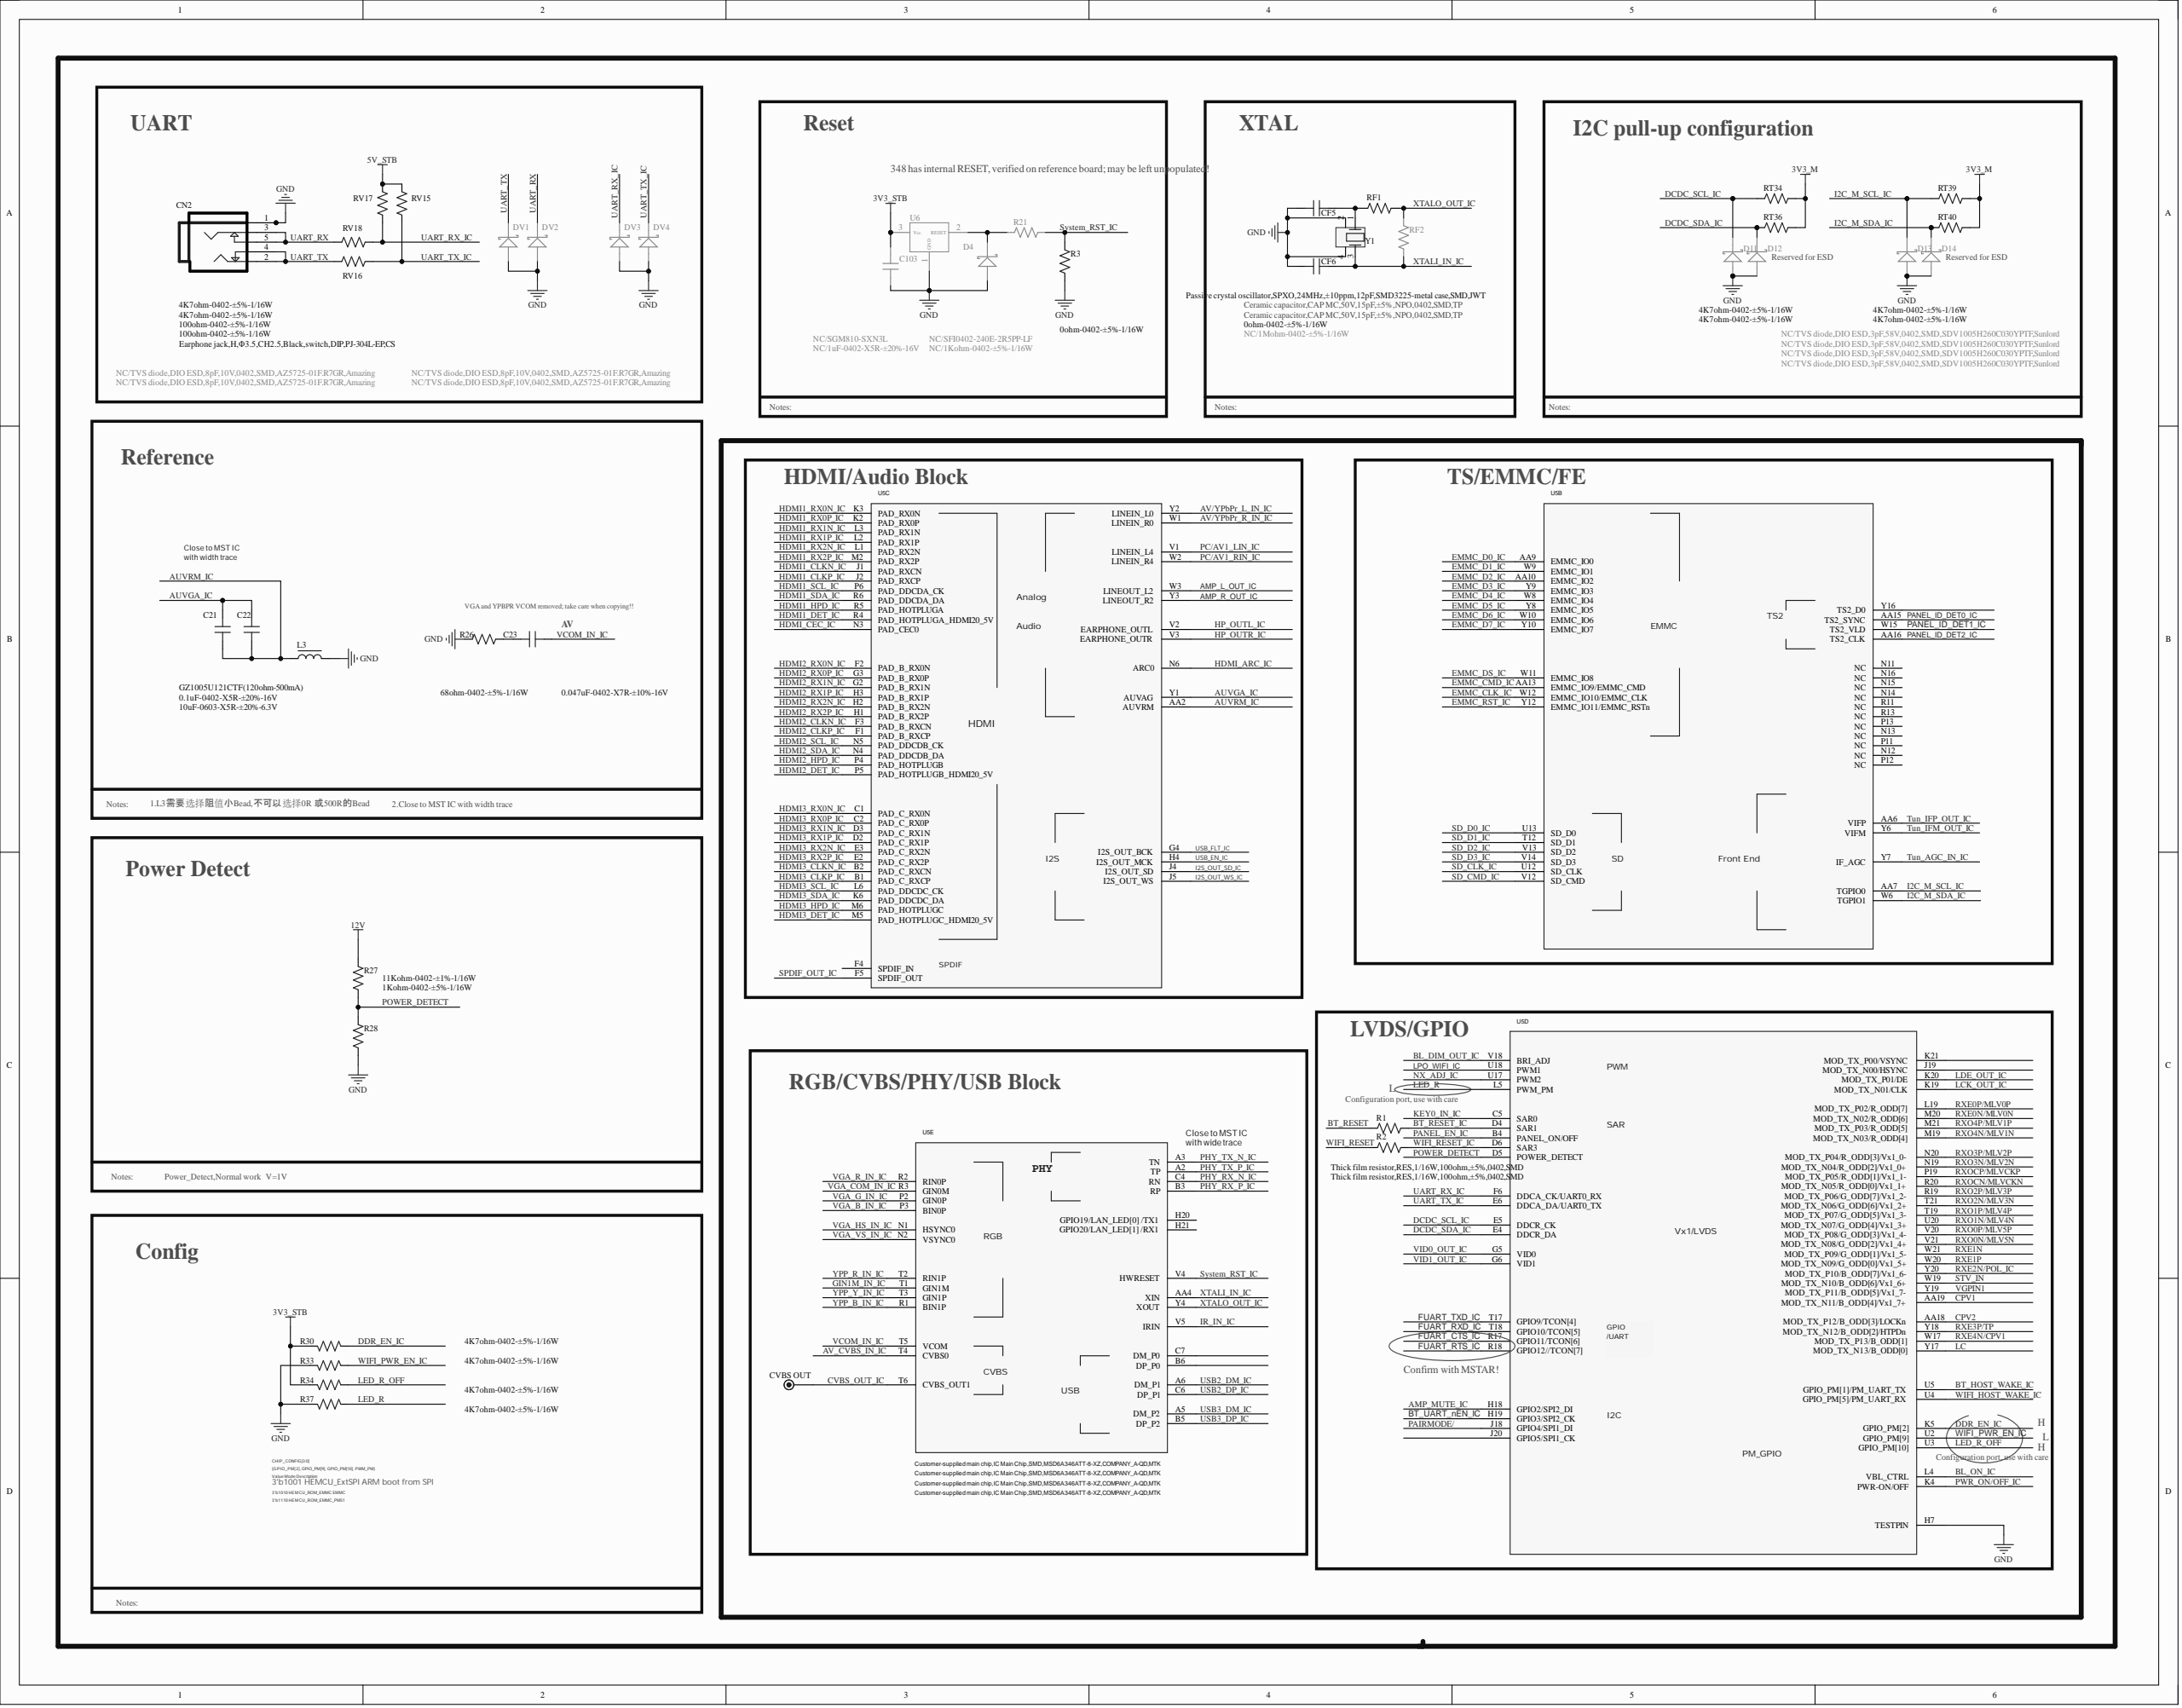Circuit board | Altium Designer | 951 parts | 509 nets | one sheet of the schematic
Parts on this sheet (reference | value | footprint):
C21 | 10uF-0603-X5R-±20%-6.3V | C0603
C22 | 0.1uF-0402-X5R-±20%-16V | C0402
C23 | 0.047uF-0402-X7R-±10%-16V | C0402
C103 | NC/1uF-0402-X5R-±20%-16V | C0402
CF5 | Ceramic capacitor,CAP MC,50V,15pF,±5%,NPO,0402,SMD,TP | C0402
CF6 | Ceramic capacitor,CAP MC,50V,15pF,±5%,NPO,0402,SMD,TP | C0402
CN2 | Earphone jack,H,F3.5,CH2.5,Black,switch,DIP,PJ-304L-EP,CS | PHONE-HD-54
D4 | NC/SFI0402-240E-2R5PP-LF | DIODE-S0402
D11 | NC/TVS diode,DIO ESD,3pF,58V,0402,SMD,SDV1005H260C030YPTF,Sunlord | DIODE-S0402
D12 | NC/TVS diode,DIO ESD,3pF,58V,0402,SMD,SDV1005H260C030YPTF,Sunlord | DIODE-S0402
D13 | NC/TVS diode,DIO ESD,3pF,58V,0402,SMD,SDV1005H260C030YPTF,Sunlord | DIODE-S0402
D14 | NC/TVS diode,DIO ESD,3pF,58V,0402,SMD,SDV1005H260C030YPTF,Sunlord | DIODE-S0402
DV1 | NC/TVS diode,DIO ESD,8pF,10V,0402,SMD,AZ5725-01F.R7GR,Amazing | DIODE-S0402
DV2 | NC/TVS diode,DIO ESD,8pF,10V,0402,SMD,AZ5725-01F.R7GR,Amazing | DIODE-S0402
DV3 | NC/TVS diode,DIO ESD,8pF,10V,0402,SMD,AZ5725-01F.R7GR,Amazing | DIODE-S0402
DV4 | NC/TVS diode,DIO ESD,8pF,10V,0402,SMD,AZ5725-01F.R7GR,Amazing | DIODE-S0402
L3 | GZ1005U121CTF(120ohm-500mA) | L0402
R1 | Thick film resistor,RES,1/16W,100ohm,±5%,0402,SMD | R0402
R2 | Thick film resistor,RES,1/16W,100ohm,±5%,0402,SMD | R0402
R3 | 0ohm-0402-±5%-1/16W | R0402
R21 | NC/1Kohm-0402-±5%-1/16W | R0402
R26 | 68ohm-0402-±5%-1/16W | R0402
R27 | 11Kohm-0402-±1%-1/16W | R0402
R28 | 1Kohm-0402-±5%-1/16W | R0402
R30 | 4K7ohm-0402-±5%-1/16W | R0402
R33 | 4K7ohm-0402-±5%-1/16W | R0402
R34 | 4K7ohm-0402-±5%-1/16W | R0402
R37 | 4K7ohm-0402-±5%-1/16W | R0402
RF1 | 0ohm-0402-±5%-1/16W | R0402
RF2 | NC/1Mohm-0402-±5%-1/16W | R0402
RT34 | 4K7ohm-0402-±5%-1/16W | R0402
RT36 | 4K7ohm-0402-±5%-1/16W | R0402
RT39 | 4K7ohm-0402-±5%-1/16W | R0402
RT40 | 4K7ohm-0402-±5%-1/16W | R0402
RV15 | 4K7ohm-0402-±5%-1/16W | R0402
RV16 | 100ohm-0402-±5%-1/16W | R0402
RV17 | 4K7ohm-0402-±5%-1/16W | R0402
RV18 | 100ohm-0402-±5%-1/16W | R0402
U5 | Customer-supplied main chip,IC Main Chip,SMD,MSD6A346ATT-8-XZ,COMPANY_A-QD,MTK | BGA406/0.8
U6 | NC/SGM810-SXN3L | SO-23-1
Y1 | Passive crystal oscillator,SPXO,24MHz,±10ppm,12pF,SMD3225-metal case,SMD,JWT | XTAL-S-3
Nets of these parts (net: part-pin ...):
XTALO_OUT_IC: RF1-2 RF2-2 U5-Y4
XTALI_IN_IC: CF6-1 RF2-1 Y1-3 U5-AA4
WIFI_RESET_IC: R2-2 U5-D6
WIFI_RESET: R2-1
WIFI_PWR_EN_IC: R33-2 U5-U2
VID0_OUT_IC: U5-G5
VCOM_IN_IC: C23-1 U5-T5
USB_FLT_IC: U5-G4
USB_EN_IC: U5-H4
USB3_DP_IC: U5-B5
USB3_DM_IC: U5-A5
USB2_DP_IC: U5-C6
USB2_DM_IC: U5-A6
UART_TX_IC: DV4-K RV15-1 RV16-1 U5-E6
UART_TX: CN2-2 CN2-4 DV1-K RV16-2
UART_RX_IC: DV3-K RV17-1 RV18-2 U5-F6
UART_RX: CN2-3 CN2-5 DV2-K RV18-1
Tun_IFP_OUT_IC: U5-AA6
Tun_IFM_OUT_IC: U5-Y6
Tun_AGC_IN_IC: U5-Y7
System_RST_IC: R3-2 R21-1 U5-V4
STV_IN: U5-W19
SPDIF_OUT_IC: U5-F5
RXOCP/MLVCKP: U5-P19
RXOCN/MLVCKN: U5-R20
RXO4P/MLV1P: U5-M21
RXO4N/MLV1N: U5-M19
RXO3P/MLV2P: U5-N20
RXO3N/MLV2N: U5-N19
RXO2P/MLV3P: U5-R19
RXO2N/MLV3N: U5-T21
RXO1P/MLV4P: U5-T19
RXO1N/MLV4N: U5-U20
RXO0P/MLV5P: U5-V20
RXO0N/MLV5N: U5-V21
RXE3P/TP: U5-Y18
RXE2N/POL_IC: U5-Y20
RXE0P/MLV0P: U5-L19
RXE0N/MLV0N: U5-M20
PWR_ON/OFF_IC: U5-K4
POWER_DETECT: R27-1 R28-2 U5-D5
PHY_TX_P_IC: U5-A2
PHY_TX_N_IC: U5-A3
PHY_RX_P_IC: U5-B3
PHY_RX_N_IC: U5-C4
PANEL_EN_IC: U5-B4
PAIRMODE/: U5-J18
NX_ADJ_IC: U5-U17
NetD4_K: D4-K R21-2 U6-2
NetCF5_1: CF5-1 RF1-1 Y1-1
NetC23_2: C23-2 R26-2
LED_R_OFF: R34-2 U5-U3
LED_R: R37-2 U5-L5
LC: U5-Y17
KEY0_IN_IC: U5-C5
IR_IN_IC: U5-V5
I2C_M_SDA_IC: D14-K RT40-1 U5-W6
I2C_M_SCL_IC: D13-K RT39-1 U5-AA7
HDMI_CEC_IC: U5-N3
HDMI_ARC_IC: U5-N6
HDMI2_SDA_IC: U5-N4
HDMI2_SCL_IC: U5-N5
HDMI2_RX2P_IC: U5-H1
HDMI2_RX2N_IC: U5-H2
HDMI2_RX1P_IC: U5-H3
HDMI2_RX1N_IC: U5-G2
HDMI2_RX0P_IC: U5-G3
HDMI2_RX0N_IC: U5-F2
HDMI2_HPD_IC: U5-P4
HDMI2_DET_IC: U5-P5
HDMI2_CLKP_IC: U5-F1
HDMI2_CLKN_IC: U5-F3
HDMI1_SDA_IC: U5-R6
HDMI1_SCL_IC: U5-P6
HDMI1_RX2P_IC: U5-M2
HDMI1_RX2N_IC: U5-L1
HDMI1_RX1P_IC: U5-L2
HDMI1_RX1N_IC: U5-L3
HDMI1_RX0P_IC: U5-K2
HDMI1_RX0N_IC: U5-K3
HDMI1_HPD_IC: U5-R5
HDMI1_DET_IC: U5-R4
HDMI1_CLKP_IC: U5-J2
HDMI1_CLKN_IC: U5-J1
GND: C103-1 CF5-2 CF6-2 CN2-1 D4-A D11-A D12-A D13-A D14-A DV1-A DV2-A DV3-A DV4-A L3-2 R3-1 R26-1 R28-1 R33-1 R37-1 U6-1 Y1-2 Y1-4 U5-D12 U5-D14 U5-H7 U5-R21 U5-U6
EMMC_RST_IC: U5-Y12
EMMC_DS_IC: U5-W11
EMMC_D7_IC: U5-Y10
EMMC_D6_IC: U5-W10
EMMC_D5_IC: U5-Y8
EMMC_D4_IC: U5-W8
EMMC_D3_IC: U5-Y9
EMMC_D2_IC: U5-AA10
EMMC_D1_IC: U5-W9
EMMC_D0_IC: U5-AA9
EMMC_CMD_IC: U5-AA13
EMMC_CLK_IC: U5-W12
DDR_EN_IC: R30-2 U5-K5
DCDC_SDA_IC: D12-K RT36-1 U5-E4
DCDC_SCL_IC: D11-K RT34-1 U5-E5
CVBS_OUT_IC: U5-T6
CPV2: U5-AA18
CPV1: U5-AA19
BT_RESET_IC: R1-2 U5-D4
BT_RESET: R1-1
BL_ON_IC: U5-L4
BL_DIM_OUT_IC: U5-V18
AV_CVBS_IN_IC: U5-T4
AV/YPbPr_R_IN_IC: U5-W1
AV/YPbPr_L_IN_IC: U5-Y2
AUVRM_IC: C21-1 C22-1 L3-1 U5-AA2
AUVGA_IC: C21-2 C22-2 U5-Y1
AMP_R_OUT_IC: U5-Y3
AMP_MUTE_IC: U5-H18
AMP_L_OUT_IC: U5-W3
12V: R27-2
5V_STB: RV15-2 RV17-2
3V3_STB: C103-2 R30-1 R34-1 U6-3
3V3_M: RT34-2 RT36-2 RT39-2 RT40-2